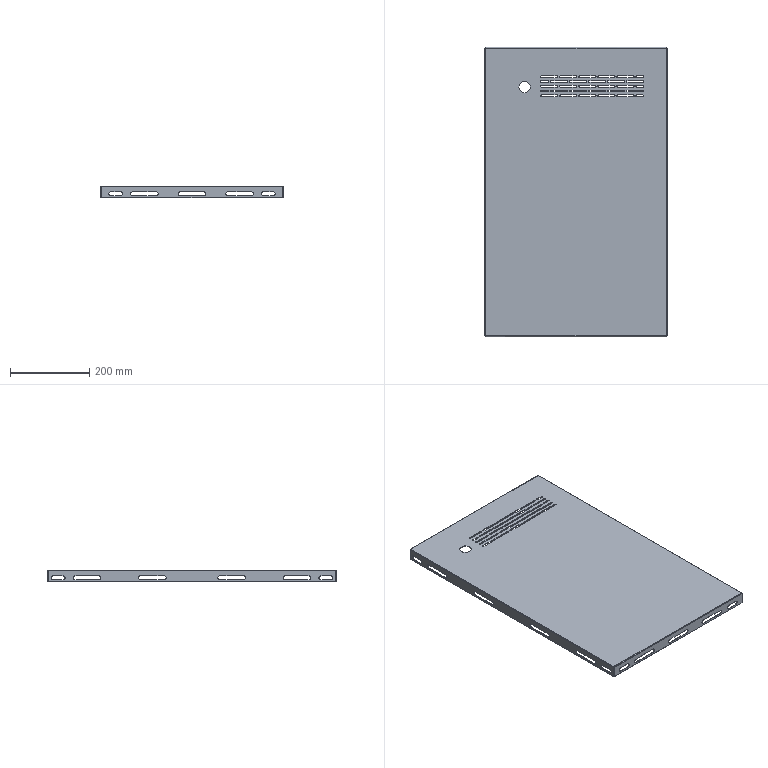Part | SolidWorks | features ICE 3, EdgeFlange 1, FlatPattern 1, SMBaseFlange 1, SheetMetal 1 | 1 solid | 280 faces | box 459 x 729 x 30 mm | volume 574629 mm3 | cylinder 145 | plane 127 | spline 8 | commonest cylinder face diameters 4 x94 10 x44 1 x4 28.5 x3